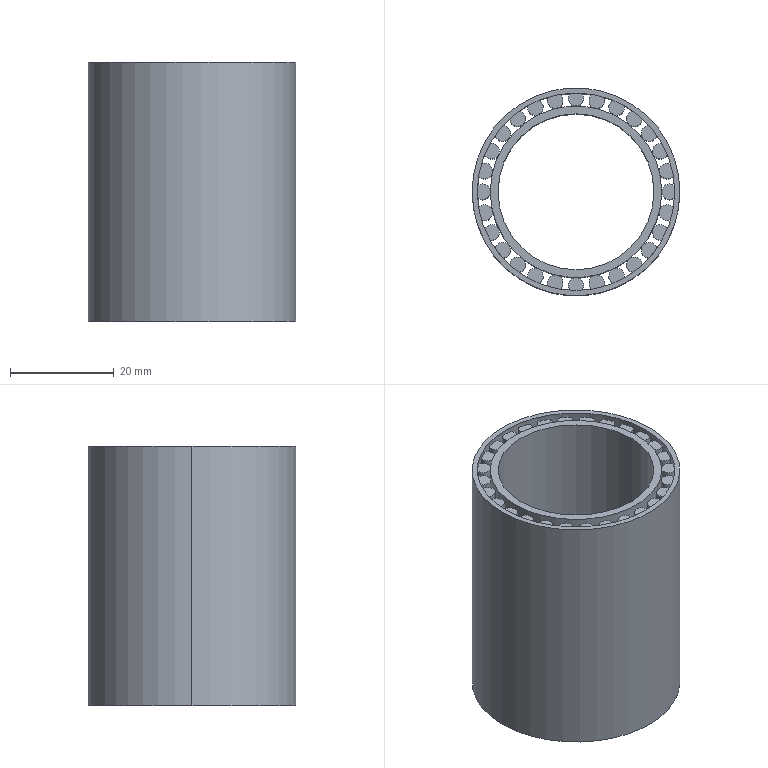Part | SolidWorks | features ICE 2, Extrusion 1 | 2 solids | 131 faces | box 40 x 40 x 50 mm | volume 21973 mm3 | cylinder 71 | plane 60 | commonest cylinder face diameters 3 x63 30 x2 33 x2 38 x2 40 x2